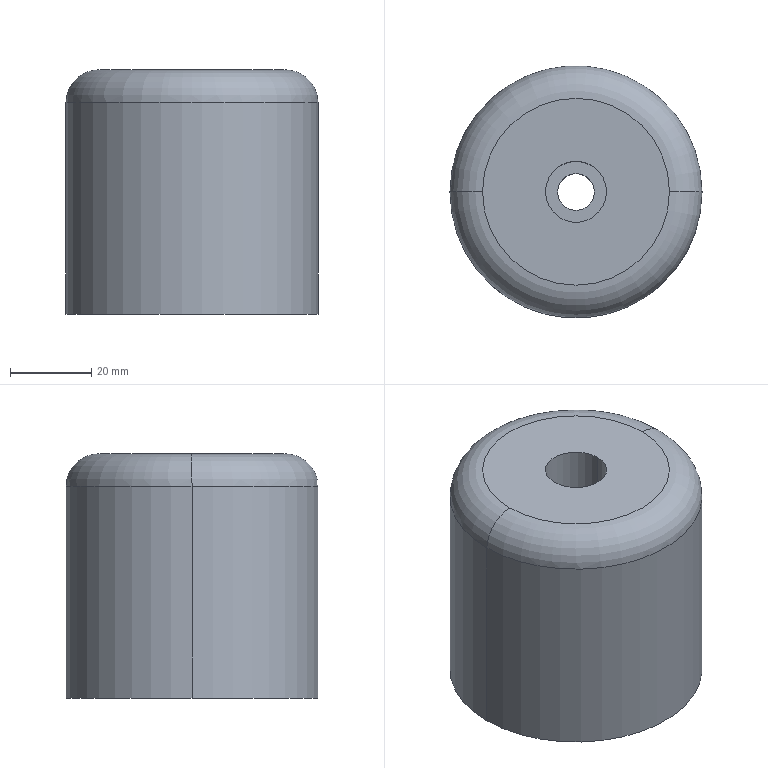Part | STEP file | 1 solid | 19 faces | box 61.9 x 61.9 x 60 mm | volume 168821 mm3 | cylinder 10 | cone 4 | plane 3 | torus 2 | commonest cylinder face diameters 6 x4 9 x2 15 x2 61.9 x2
STEP:
#1=CARTESIAN_POINT('',(0.,0.,0.));
#2=DIRECTION('',(0.,0.,1.));
#3=DIRECTION('',(1.,0.,0.));
#4=AXIS2_PLACEMENT_3D('',#1,#2,#3);
#5=CARTESIAN_POINT('',(-30.95,0.,22.));
#6=VERTEX_POINT('',#5);
#7=CARTESIAN_POINT('',(30.95,0.,22.));
#8=VERTEX_POINT('',#7);
#9=CARTESIAN_POINT('',(0.,0.,22.));
#10=DIRECTION('',(0.,0.,-1.));
#11=DIRECTION('',(1.,0.,0.));
#12=AXIS2_PLACEMENT_3D('',#9,#10,#11);
#13=CIRCLE('',#12,30.95);
#14=CARTESIAN_POINT('',(0.,0.,22.));
#15=DIRECTION('',(0.,0.,1.));
#16=DIRECTION('',(1.,0.,0.));
#17=AXIS2_PLACEMENT_3D('',#14,#15,#16);
#18=TOROIDAL_SURFACE('',#17,22.95,8.);
#19=CARTESIAN_POINT('',(6.283,0.));
#20=DIRECTION('',(-1.,0.));
#21=VECTOR('',#20,1.);
#22=LINE('',#19,#21);
#23=(GEOMETRIC_REPRESENTATION_CONTEXT(2)PARAMETRIC_REPRESENTATION_CONTEXT()REPRESENTATION_CONTEXT('',''));
#24=DEFINITIONAL_REPRESENTATION('',(#22),#23);
#25=PCURVE('',#18,#24);
#26=CARTESIAN_POINT('',(0.,0.,30.));
#27=DIRECTION('',(0.,0.,-1.));
#28=DIRECTION('',(-1.,0.,0.));
#29=AXIS2_PLACEMENT_3D('',#26,#27,#28);
#30=CYLINDRICAL_SURFACE('',#29,30.95);
#31=CARTESIAN_POINT('',(-3.142,8.));
#32=DIRECTION('',(1.,0.));
#33=VECTOR('',#32,1.);
#34=LINE('',#31,#33);
#35=(GEOMETRIC_REPRESENTATION_CONTEXT(2)PARAMETRIC_REPRESENTATION_CONTEXT()REPRESENTATION_CONTEXT('',''));
#36=DEFINITIONAL_REPRESENTATION('',(#34),#35);
#37=PCURVE('',#30,#36);
#38=SURFACE_CURVE('',#13,(#25,#37),.PCURVE_S1.);
#39=EDGE_CURVE('',#6,#8,#38,.T.);
#40=ORIENTED_EDGE('',*,*,#39,.F.);
#41=CARTESIAN_POINT('',(-22.95,0.,30.));
#42=VERTEX_POINT('',#41);
#43=CARTESIAN_POINT('',(-22.95,0.,22.));
#44=DIRECTION('',(0.,1.,0.));
#45=DIRECTION('',(-1.,0.,0.));
#46=AXIS2_PLACEMENT_3D('',#43,#44,#45);
#47=CIRCLE('',#46,8.);
#48=CARTESIAN_POINT('',(3.142,0.));
#49=DIRECTION('',(0.,1.));
#50=VECTOR('',#49,1.);
#51=LINE('',#48,#50);
#52=(GEOMETRIC_REPRESENTATION_CONTEXT(2)PARAMETRIC_REPRESENTATION_CONTEXT()REPRESENTATION_CONTEXT('',''));
#53=DEFINITIONAL_REPRESENTATION('',(#51),#52);
#54=PCURVE('',#18,#53);
#55=CARTESIAN_POINT('',(0.,0.,22.));
#56=DIRECTION('',(0.,0.,1.));
#57=DIRECTION('',(1.,0.,0.));
#58=AXIS2_PLACEMENT_3D('',#55,#56,#57);
#59=TOROIDAL_SURFACE('',#58,22.95,8.);
#60=CARTESIAN_POINT('',(3.142,0.));
#61=DIRECTION('',(0.,1.));
#62=VECTOR('',#61,1.);
#63=LINE('',#60,#62);
#64=(GEOMETRIC_REPRESENTATION_CONTEXT(2)PARAMETRIC_REPRESENTATION_CONTEXT()REPRESENTATION_CONTEXT('',''));
#65=DEFINITIONAL_REPRESENTATION('',(#63),#64);
#66=PCURVE('',#59,#65);
#67=SURFACE_CURVE('',#47,(#54,#66),.PCURVE_S1.);
#68=EDGE_CURVE('',#6,#42,#67,.T.);
#69=ORIENTED_EDGE('',*,*,#68,.T.);
#70=CARTESIAN_POINT('',(22.95,0.,30.));
#71=VERTEX_POINT('',#70);
#72=CARTESIAN_POINT('',(0.,0.,30.));
#73=DIRECTION('',(0.,0.,1.));
#74=DIRECTION('',(1.,0.,0.));
#75=AXIS2_PLACEMENT_3D('',#72,#73,#74);
#76=CIRCLE('',#75,22.95);
#77=CARTESIAN_POINT('',(0.,1.571));
#78=DIRECTION('',(1.,0.));
#79=VECTOR('',#78,1.);
#80=LINE('',#77,#79);
#81=(GEOMETRIC_REPRESENTATION_CONTEXT(2)PARAMETRIC_REPRESENTATION_CONTEXT()REPRESENTATION_CONTEXT('',''));
#82=DEFINITIONAL_REPRESENTATION('',(#80),#81);
#83=PCURVE('',#18,#82);
#84=CARTESIAN_POINT('',(0.,0.,30.));
#85=DIRECTION('',(0.,0.,1.));
#86=DIRECTION('',(1.,0.,0.));
#87=AXIS2_PLACEMENT_3D('',#84,#85,#86);
#88=PLANE('',#87);
#89=CARTESIAN_POINT('',(0.,0.));
#90=DIRECTION('',(1.,0.));
#91=AXIS2_PLACEMENT_2D('',#89,#90);
#92=CIRCLE('',#91,22.95);
#93=(GEOMETRIC_REPRESENTATION_CONTEXT(2)PARAMETRIC_REPRESENTATION_CONTEXT()REPRESENTATION_CONTEXT('',''));
#94=DEFINITIONAL_REPRESENTATION('',(#92),#93);
#95=PCURVE('',#88,#94);
#96=SURFACE_CURVE('',#76,(#83,#95),.PCURVE_S1.);
#97=EDGE_CURVE('',#71,#42,#96,.T.);
#98=ORIENTED_EDGE('',*,*,#97,.F.);
#99=CARTESIAN_POINT('',(22.95,0.,22.));
#100=DIRECTION('',(0.,-1.,0.));
#101=DIRECTION('',(0.,0.,-1.));
#102=AXIS2_PLACEMENT_3D('',#99,#100,#101);
#103=CIRCLE('',#102,8.);
#104=CARTESIAN_POINT('',(0.,-1.571));
#105=DIRECTION('',(0.,1.));
#106=VECTOR('',#105,1.);
#107=LINE('',#104,#106);
#108=(GEOMETRIC_REPRESENTATION_CONTEXT(2)PARAMETRIC_REPRESENTATION_CONTEXT()REPRESENTATION_CONTEXT('',''));
#109=DEFINITIONAL_REPRESENTATION('',(#107),#108);
#110=PCURVE('',#18,#109);
#111=CARTESIAN_POINT('',(6.283,-1.571));
#112=DIRECTION('',(0.,1.));
#113=VECTOR('',#112,1.);
#114=LINE('',#111,#113);
#115=(GEOMETRIC_REPRESENTATION_CONTEXT(2)PARAMETRIC_REPRESENTATION_CONTEXT()REPRESENTATION_CONTEXT('',''));
#116=DEFINITIONAL_REPRESENTATION('',(#114),#115);
#117=PCURVE('',#59,#116);
#118=SURFACE_CURVE('',#103,(#110,#117),.PCURVE_S1.);
#119=EDGE_CURVE('',#8,#71,#118,.T.);
#120=ORIENTED_EDGE('',*,*,#119,.F.);
#121=EDGE_LOOP('',(#40,#69,#98,#120));
#122=FACE_BOUND('',#121,.T.);
#123=ADVANCED_FACE('',(#122),#18,.T.);
#124=CARTESIAN_POINT('',(7.5,0.,-10.));
#125=VERTEX_POINT('',#124);
#126=CARTESIAN_POINT('',(7.5,0.,30.));
#127=VERTEX_POINT('',#126);
#128=CARTESIAN_POINT('',(7.5,0.,30.));
#129=DIRECTION('',(0.,0.,1.));
#130=VECTOR('',#129,1.);
#131=LINE('',#128,#130);
#132=CARTESIAN_POINT('',(0.,0.,30.));
#133=DIRECTION('',(0.,0.,1.));
#134=DIRECTION('',(1.,0.,0.));
#135=AXIS2_PLACEMENT_3D('',#132,#133,#134);
#136=CYLINDRICAL_SURFACE('',#135,7.5);
#137=CARTESIAN_POINT('',(6.283,0.));
#138=DIRECTION('',(0.,1.));
#139=VECTOR('',#138,1.);
#140=LINE('',#137,#139);
#141=(GEOMETRIC_REPRESENTATION_CONTEXT(2)PARAMETRIC_REPRESENTATION_CONTEXT()REPRESENTATION_CONTEXT('',''));
#142=DEFINITIONAL_REPRESENTATION('',(#140),#141);
#143=PCURVE('',#136,#142);
#144=CARTESIAN_POINT('',(0.,0.,30.));
#145=DIRECTION('',(0.,0.,1.));
#146=DIRECTION('',(1.,0.,0.));
#147=AXIS2_PLACEMENT_3D('',#144,#145,#146);
#148=CYLINDRICAL_SURFACE('',#147,7.5);
#149=CARTESIAN_POINT('',(0.,0.));
#150=DIRECTION('',(0.,1.));
#151=VECTOR('',#150,1.);
#152=LINE('',#149,#151);
#153=(GEOMETRIC_REPRESENTATION_CONTEXT(2)PARAMETRIC_REPRESENTATION_CONTEXT()REPRESENTATION_CONTEXT('',''));
#154=DEFINITIONAL_REPRESENTATION('',(#152),#153);
#155=PCURVE('',#148,#154);
#156=SURFACE_CURVE('',#131,(#143,#155),.PCURVE_S1.);
#157=EDGE_CURVE('',#125,#127,#156,.T.);
#158=ORIENTED_EDGE('',*,*,#157,.T.);
#159=CARTESIAN_POINT('',(-7.5,0.,30.));
#160=VERTEX_POINT('',#159);
#161=CARTESIAN_POINT('',(0.,0.,30.));
#162=DIRECTION('',(0.,0.,1.));
#163=DIRECTION('',(1.,0.,0.));
#164=AXIS2_PLACEMENT_3D('',#161,#162,#163);
#165=CIRCLE('',#164,7.5);
#166=CARTESIAN_POINT('',(0.,0.));
#167=DIRECTION('',(1.,0.));
#168=VECTOR('',#167,1.);
#169=LINE('',#166,#168);
#170=(GEOMETRIC_REPRESENTATION_CONTEXT(2)PARAMETRIC_REPRESENTATION_CONTEXT()REPRESENTATION_CONTEXT('',''));
#171=DEFINITIONAL_REPRESENTATION('',(#169),#170);
#172=PCURVE('',#136,#171);
#173=CARTESIAN_POINT('',(0.,0.));
#174=DIRECTION('',(1.,0.));
#175=AXIS2_PLACEMENT_2D('',#173,#174);
#176=CIRCLE('',#175,7.5);
#177=(GEOMETRIC_REPRESENTATION_CONTEXT(2)PARAMETRIC_REPRESENTATION_CONTEXT()REPRESENTATION_CONTEXT('',''));
#178=DEFINITIONAL_REPRESENTATION('',(#176),#177);
#179=PCURVE('',#88,#178);
#180=SURFACE_CURVE('',#165,(#172,#179),.PCURVE_S1.);
#181=EDGE_CURVE('',#160,#127,#180,.T.);
#182=ORIENTED_EDGE('',*,*,#181,.F.);
#183=CARTESIAN_POINT('',(-7.5,0.,-10.));
#184=VERTEX_POINT('',#183);
#185=CARTESIAN_POINT('',(-7.5,0.,30.));
#186=DIRECTION('',(0.,0.,1.));
#187=VECTOR('',#186,1.);
#188=LINE('',#185,#187);
#189=CARTESIAN_POINT('',(3.142,0.));
#190=DIRECTION('',(0.,1.));
#191=VECTOR('',#190,1.);
#192=LINE('',#189,#191);
#193=(GEOMETRIC_REPRESENTATION_CONTEXT(2)PARAMETRIC_REPRESENTATION_CONTEXT()REPRESENTATION_CONTEXT('',''));
#194=DEFINITIONAL_REPRESENTATION('',(#192),#193);
#195=PCURVE('',#136,#194);
#196=CARTESIAN_POINT('',(3.142,0.));
#197=DIRECTION('',(0.,1.));
#198=VECTOR('',#197,1.);
#199=LINE('',#196,#198);
#200=(GEOMETRIC_REPRESENTATION_CONTEXT(2)PARAMETRIC_REPRESENTATION_CONTEXT()REPRESENTATION_CONTEXT('',''));
#201=DEFINITIONAL_REPRESENTATION('',(#199),#200);
#202=PCURVE('',#148,#201);
#203=SURFACE_CURVE('',#188,(#195,#202),.PCURVE_S1.);
#204=EDGE_CURVE('',#184,#160,#203,.T.);
#205=ORIENTED_EDGE('',*,*,#204,.F.);
#206=CARTESIAN_POINT('',(0.,0.,-10.));
#207=DIRECTION('',(0.,0.,1.));
#208=DIRECTION('',(1.,0.,0.));
#209=AXIS2_PLACEMENT_3D('',#206,#207,#208);
#210=CIRCLE('',#209,7.5);
#211=CARTESIAN_POINT('',(0.,-40.));
#212=DIRECTION('',(1.,0.));
#213=VECTOR('',#212,1.);
#214=LINE('',#211,#213);
#215=(GEOMETRIC_REPRESENTATION_CONTEXT(2)PARAMETRIC_REPRESENTATION_CONTEXT()REPRESENTATION_CONTEXT('',''));
#216=DEFINITIONAL_REPRESENTATION('',(#214),#215);
#217=PCURVE('',#136,#216);
#218=CARTESIAN_POINT('',(4.5,0.,-10.));
#219=DIRECTION('',(0.,0.,-1.));
#220=DIRECTION('',(-1.,0.,0.));
#221=AXIS2_PLACEMENT_3D('',#218,#219,#220);
#222=PLANE('',#221);
#223=CARTESIAN_POINT('',(-3.,0.));
#224=CARTESIAN_POINT('',(-3.,12.99));
#225=CARTESIAN_POINT('',(8.25,6.495));
#226=CARTESIAN_POINT('',(19.5,0.));
#227=CARTESIAN_POINT('',(8.25,-6.495));
#228=CARTESIAN_POINT('',(-3.,-12.99));
#229=CARTESIAN_POINT('',(-3.,0.));
#230=(BOUNDED_CURVE()B_SPLINE_CURVE(2,(#223,#224,#225,#226,#227,#228,#229),.UNSPECIFIED.,.T.,.F.)B_SPLINE_CURVE_WITH_KNOTS((1,2,2,2,2,1),(-2.094,0.,2.094,4.189,6.283,8.378),.UNSPECIFIED.)CURVE()GEOMETRIC_REPRESENTATION_ITEM()RATIONAL_B_SPLINE_CURVE((1.,0.5,1.,0.5,1.,0.5,1.))REPRESENTATION_ITEM(''));
#231=(GEOMETRIC_REPRESENTATION_CONTEXT(2)PARAMETRIC_REPRESENTATION_CONTEXT()REPRESENTATION_CONTEXT('',''));
#232=DEFINITIONAL_REPRESENTATION('',(#230),#231);
#233=PCURVE('',#222,#232);
#234=SURFACE_CURVE('',#210,(#217,#233),.PCURVE_S1.);
#235=EDGE_CURVE('',#184,#125,#234,.T.);
#236=ORIENTED_EDGE('',*,*,#235,.T.);
#237=EDGE_LOOP('',(#158,#182,#205,#236));
#238=FACE_BOUND('',#237,.F.);
#239=ADVANCED_FACE('',(#238),#136,.F.);
#240=CARTESIAN_POINT('',(4.5,0.,-30.));
#241=VERTEX_POINT('',#240);
#242=CARTESIAN_POINT('',(4.5,0.,-10.));
#243=VERTEX_POINT('',#242);
#244=CARTESIAN_POINT('',(4.5,0.,30.));
#245=DIRECTION('',(0.,0.,1.));
#246=VECTOR('',#245,1.);
#247=LINE('',#244,#246);
#248=CARTESIAN_POINT('',(0.,0.,30.));
#249=DIRECTION('',(0.,0.,1.));
#250=DIRECTION('',(1.,0.,0.));
#251=AXIS2_PLACEMENT_3D('',#248,#249,#250);
#252=CYLINDRICAL_SURFACE('',#251,4.5);
#253=CARTESIAN_POINT('',(6.283,0.));
#254=DIRECTION('',(0.,1.));
#255=VECTOR('',#254,1.);
#256=LINE('',#253,#255);
#257=(GEOMETRIC_REPRESENTATION_CONTEXT(2)PARAMETRIC_REPRESENTATION_CONTEXT()REPRESENTATION_CONTEXT('',''));
#258=DEFINITIONAL_REPRESENTATION('',(#256),#257);
#259=PCURVE('',#252,#258);
#260=CARTESIAN_POINT('',(0.,0.,30.));
#261=DIRECTION('',(0.,0.,1.));
#262=DIRECTION('',(1.,0.,0.));
#263=AXIS2_PLACEMENT_3D('',#260,#261,#262);
#264=CYLINDRICAL_SURFACE('',#263,4.5);
#265=CARTESIAN_POINT('',(0.,0.));
#266=DIRECTION('',(0.,1.));
#267=VECTOR('',#266,1.);
#268=LINE('',#265,#267);
#269=(GEOMETRIC_REPRESENTATION_CONTEXT(2)PARAMETRIC_REPRESENTATION_CONTEXT()REPRESENTATION_CONTEXT('',''));
#270=DEFINITIONAL_REPRESENTATION('',(#268),#269);
#271=PCURVE('',#264,#270);
#272=SURFACE_CURVE('',#247,(#259,#271),.PCURVE_S1.);
#273=EDGE_CURVE('',#241,#243,#272,.T.);
#274=ORIENTED_EDGE('',*,*,#273,.T.);
#275=CARTESIAN_POINT('',(-4.5,0.,-10.));
#276=VERTEX_POINT('',#275);
#277=CARTESIAN_POINT('',(0.,0.,-10.));
#278=DIRECTION('',(0.,0.,1.));
#279=DIRECTION('',(1.,0.,0.));
#280=AXIS2_PLACEMENT_3D('',#277,#278,#279);
#281=CIRCLE('',#280,4.5);
#282=CARTESIAN_POINT('',(0.,-40.));
#283=DIRECTION('',(1.,0.));
#284=VECTOR('',#283,1.);
#285=LINE('',#282,#284);
#286=(GEOMETRIC_REPRESENTATION_CONTEXT(2)PARAMETRIC_REPRESENTATION_CONTEXT()REPRESENTATION_CONTEXT('',''));
#287=DEFINITIONAL_REPRESENTATION('',(#285),#286);
#288=PCURVE('',#252,#287);
#289=CARTESIAN_POINT('',(0.,0.));
#290=CARTESIAN_POINT('',(0.,7.794));
#291=CARTESIAN_POINT('',(6.75,3.897));
#292=CARTESIAN_POINT('',(13.5,0.));
#293=CARTESIAN_POINT('',(6.75,-3.897));
#294=CARTESIAN_POINT('',(0.,-7.794));
#295=CARTESIAN_POINT('',(0.,0.));
#296=(BOUNDED_CURVE()B_SPLINE_CURVE(2,(#289,#290,#291,#292,#293,#294,#295),.UNSPECIFIED.,.T.,.F.)B_SPLINE_CURVE_WITH_KNOTS((1,2,2,2,2,1),(-2.094,0.,2.094,4.189,6.283,8.378),.UNSPECIFIED.)CURVE()GEOMETRIC_REPRESENTATION_ITEM()RATIONAL_B_SPLINE_CURVE((1.,0.5,1.,0.5,1.,0.5,1.))REPRESENTATION_ITEM(''));
#297=(GEOMETRIC_REPRESENTATION_CONTEXT(2)PARAMETRIC_REPRESENTATION_CONTEXT()REPRESENTATION_CONTEXT('',''));
#298=DEFINITIONAL_REPRESENTATION('',(#296),#297);
#299=PCURVE('',#222,#298);
#300=SURFACE_CURVE('',#281,(#288,#299),.PCURVE_S1.);
#301=EDGE_CURVE('',#276,#243,#300,.T.);
#302=ORIENTED_EDGE('',*,*,#301,.F.);
#303=CARTESIAN_POINT('',(-4.5,0.,-30.));
#304=VERTEX_POINT('',#303);
#305=CARTESIAN_POINT('',(-4.5,0.,30.));
#306=DIRECTION('',(0.,0.,1.));
#307=VECTOR('',#306,1.);
#308=LINE('',#305,#307);
#309=CARTESIAN_POINT('',(3.142,0.));
#310=DIRECTION('',(0.,1.));
#311=VECTOR('',#310,1.);
#312=LINE('',#309,#311);
#313=(GEOMETRIC_REPRESENTATION_CONTEXT(2)PARAMETRIC_REPRESENTATION_CONTEXT()REPRESENTATION_CONTEXT('',''));
#314=DEFINITIONAL_REPRESENTATION('',(#312),#313);
#315=PCURVE('',#252,#314);
#316=CARTESIAN_POINT('',(3.142,0.));
#317=DIRECTION('',(0.,1.));
#318=VECTOR('',#317,1.);
#319=LINE('',#316,#318);
#320=(GEOMETRIC_REPRESENTATION_CONTEXT(2)PARAMETRIC_REPRESENTATION_CONTEXT()REPRESENTATION_CONTEXT('',''));
#321=DEFINITIONAL_REPRESENTATION('',(#319),#320);
#322=PCURVE('',#264,#321);
#323=SURFACE_CURVE('',#308,(#315,#322),.PCURVE_S1.);
#324=EDGE_CURVE('',#304,#276,#323,.T.);
#325=ORIENTED_EDGE('',*,*,#324,.F.);
#326=CARTESIAN_POINT('',(0.,0.,-30.));
#327=DIRECTION('',(0.,0.,1.));
#328=DIRECTION('',(1.,0.,0.));
#329=AXIS2_PLACEMENT_3D('',#326,#327,#328);
#330=CIRCLE('',#329,4.5);
#331=CARTESIAN_POINT('',(0.,-60.));
#332=DIRECTION('',(1.,0.));
#333=VECTOR('',#332,1.);
#334=LINE('',#331,#333);
#335=(GEOMETRIC_REPRESENTATION_CONTEXT(2)PARAMETRIC_REPRESENTATION_CONTEXT()REPRESENTATION_CONTEXT('',''));
#336=DEFINITIONAL_REPRESENTATION('',(#334),#335);
#337=PCURVE('',#252,#336);
#338=CARTESIAN_POINT('',(0.,0.,-30.));
#339=DIRECTION('',(0.,0.,1.));
#340=DIRECTION('',(1.,0.,0.));
#341=AXIS2_PLACEMENT_3D('',#338,#339,#340);
#342=PLANE('',#341);
#343=CARTESIAN_POINT('',(0.,0.));
#344=DIRECTION('',(1.,0.));
#345=AXIS2_PLACEMENT_2D('',#343,#344);
#346=CIRCLE('',#345,4.5);
#347=(GEOMETRIC_REPRESENTATION_CONTEXT(2)PARAMETRIC_REPRESENTATION_CONTEXT()REPRESENTATION_CONTEXT('',''));
#348=DEFINITIONAL_REPRESENTATION('',(#346),#347);
#349=PCURVE('',#342,#348);
#350=SURFACE_CURVE('',#330,(#337,#349),.PCURVE_S1.);
#351=EDGE_CURVE('',#304,#241,#350,.T.);
#352=ORIENTED_EDGE('',*,*,#351,.T.);
#353=EDGE_LOOP('',(#274,#302,#325,#352));
#354=FACE_BOUND('',#353,.F.);
#355=ADVANCED_FACE('',(#354),#252,.F.);
#356=CARTESIAN_POINT('',(17.,0.,-15.));
#357=VERTEX_POINT('',#356);
#358=CARTESIAN_POINT('',(17.,0.,-30.));
#359=VERTEX_POINT('',#358);
#360=CARTESIAN_POINT('',(17.,0.,-30.));
#361=DIRECTION('',(0.,0.,-1.));
#362=VECTOR('',#361,1.);
#363=LINE('',#360,#362);
#364=CARTESIAN_POINT('',(20.,0.,-30.));
#365=DIRECTION('',(0.,0.,-1.));
#366=DIRECTION('',(-1.,0.,0.));
#367=AXIS2_PLACEMENT_3D('',#364,#365,#366);
#368=CYLINDRICAL_SURFACE('',#367,3.);
#369=CARTESIAN_POINT('',(6.283,0.));
#370=DIRECTION('',(0.,1.));
#371=VECTOR('',#370,1.);
#372=LINE('',#369,#371);
#373=(GEOMETRIC_REPRESENTATION_CONTEXT(2)PARAMETRIC_REPRESENTATION_CONTEXT()REPRESENTATION_CONTEXT('',''));
#374=DEFINITIONAL_REPRESENTATION('',(#372),#373);
#375=PCURVE('',#368,#374);
#376=CARTESIAN_POINT('',(20.,0.,-30.));
#377=DIRECTION('',(0.,0.,-1.));
#378=DIRECTION('',(-1.,0.,0.));
#379=AXIS2_PLACEMENT_3D('',#376,#377,#378);
#380=CYLINDRICAL_SURFACE('',#379,3.);
#381=CARTESIAN_POINT('',(0.,0.));
#382=DIRECTION('',(0.,1.));
#383=VECTOR('',#382,1.);
#384=LINE('',#381,#383);
#385=(GEOMETRIC_REPRESENTATION_CONTEXT(2)PARAMETRIC_REPRESENTATION_CONTEXT()REPRESENTATION_CONTEXT('',''));
#386=DEFINITIONAL_REPRESENTATION('',(#384),#385);
#387=PCURVE('',#380,#386);
#388=SURFACE_CURVE('',#363,(#375,#387),.PCURVE_S1.);
#389=EDGE_CURVE('',#357,#359,#388,.T.);
#390=ORIENTED_EDGE('',*,*,#389,.T.);
#391=CARTESIAN_POINT('',(23.,0.,-30.));
#392=VERTEX_POINT('',#391);
#393=CARTESIAN_POINT('',(20.,0.,-30.));
#394=DIRECTION('',(0.,0.,-1.));
#395=DIRECTION('',(-1.,0.,0.));
#396=AXIS2_PLACEMENT_3D('',#393,#394,#395);
#397=CIRCLE('',#396,3.);
#398=CARTESIAN_POINT('',(0.,0.));
#399=DIRECTION('',(1.,0.));
#400=VECTOR('',#399,1.);
#401=LINE('',#398,#400);
#402=(GEOMETRIC_REPRESENTATION_CONTEXT(2)PARAMETRIC_REPRESENTATION_CONTEXT()REPRESENTATION_CONTEXT('',''));
#403=DEFINITIONAL_REPRESENTATION('',(#401),#402);
#404=PCURVE('',#368,#403);
#405=CARTESIAN_POINT('',(17.,0.));
#406=CARTESIAN_POINT('',(17.,5.196));
#407=CARTESIAN_POINT('',(21.5,2.598));
#408=CARTESIAN_POINT('',(26.,0.));
#409=CARTESIAN_POINT('',(21.5,-2.598));
#410=CARTESIAN_POINT('',(17.,-5.196));
#411=CARTESIAN_POINT('',(17.,0.));
#412=(BOUNDED_CURVE()B_SPLINE_CURVE(2,(#405,#406,#407,#408,#409,#410,#411),.UNSPECIFIED.,.T.,.F.)B_SPLINE_CURVE_WITH_KNOTS((1,2,2,2,2,1),(-2.094,0.,2.094,4.189,6.283,8.378),.UNSPECIFIED.)CURVE()GEOMETRIC_REPRESENTATION_ITEM()RATIONAL_B_SPLINE_CURVE((1.,0.5,1.,0.5,1.,0.5,1.))REPRESENTATION_ITEM(''));
#413=(GEOMETRIC_REPRESENTATION_CONTEXT(2)PARAMETRIC_REPRESENTATION_CONTEXT()REPRESENTATION_CONTEXT('',''));
#414=DEFINITIONAL_REPRESENTATION('',(#412),#413);
#415=PCURVE('',#342,#414);
#416=SURFACE_CURVE('',#397,(#404,#415),.PCURVE_S1.);
#417=EDGE_CURVE('',#392,#359,#416,.T.);
#418=ORIENTED_EDGE('',*,*,#417,.F.);
#419=CARTESIAN_POINT('',(23.,0.,-15.));
#420=VERTEX_POINT('',#419);
#421=CARTESIAN_POINT('',(23.,0.,-30.));
#422=DIRECTION('',(0.,0.,-1.));
#423=VECTOR('',#422,1.);
#424=LINE('',#421,#423);
#425=CARTESIAN_POINT('',(3.142,0.));
#426=DIRECTION('',(0.,1.));
#427=VECTOR('',#426,1.);
#428=LINE('',#425,#427);
#429=(GEOMETRIC_REPRESENTATION_CONTEXT(2)PARAMETRIC_REPRESENTATION_CONTEXT()REPRESENTATION_CONTEXT('',''));
#430=DEFINITIONAL_REPRESENTATION('',(#428),#429);
#431=PCURVE('',#368,#430);
#432=CARTESIAN_POINT('',(3.142,0.));
#433=DIRECTION('',(0.,1.));
#434=VECTOR('',#433,1.);
#435=LINE('',#432,#434);
#436=(GEOMETRIC_REPRESENTATION_CONTEXT(2)PARAMETRIC_REPRESENTATION_CONTEXT()REPRESENTATION_CONTEXT('',''));
#437=DEFINITIONAL_REPRESENTATION('',(#435),#436);
#438=PCURVE('',#380,#437);
#439=SURFACE_CURVE('',#424,(#431,#438),.PCURVE_S1.);
#440=EDGE_CURVE('',#420,#392,#439,.T.);
#441=ORIENTED_EDGE('',*,*,#440,.F.);
#442=CARTESIAN_POINT('',(20.,0.,-15.));
#443=DIRECTION('',(0.,0.,-1.));
#444=DIRECTION('',(-1.,0.,0.));
#445=AXIS2_PLACEMENT_3D('',#442,#443,#444);
#446=CIRCLE('',#445,3.);
#447=CARTESIAN_POINT('',(0.,-15.));
#448=DIRECTION('',(1.,0.));
#449=VECTOR('',#448,1.);
#450=LINE('',#447,#449);
#451=(GEOMETRIC_REPRESENTATION_CONTEXT(2)PARAMETRIC_REPRESENTATION_CONTEXT()REPRESENTATION_CONTEXT('',''));
#452=DEFINITIONAL_REPRESENTATION('',(#450),#451);
#453=PCURVE('',#368,#452);
#454=CARTESIAN_POINT('',(20.,0.,-15.));
#455=DIRECTION('',(0.,0.,-1.));
#456=DIRECTION('',(-1.,0.,0.));
#457=AXIS2_PLACEMENT_3D('',#454,#455,#456);
#458=CONICAL_SURFACE('',#457,3.,1.03);
#459=CARTESIAN_POINT('',(0.,0.));
#460=DIRECTION('',(1.,0.));
#461=VECTOR('',#460,1.);
#462=LINE('',#459,#461);
#463=(GEOMETRIC_REPRESENTATION_CONTEXT(2)PARAMETRIC_REPRESENTATION_CONTEXT()REPRESENTATION_CONTEXT('',''));
#464=DEFINITIONAL_REPRESENTATION('',(#462),#463);
#465=PCURVE('',#458,#464);
#466=SURFACE_CURVE('',#446,(#453,#465),.PCURVE_S1.);
#467=EDGE_CURVE('',#420,#357,#466,.T.);
#468=ORIENTED_EDGE('',*,*,#467,.T.);
#469=EDGE_LOOP('',(#390,#418,#441,#468));
#470=FACE_BOUND('',#469,.F.);
#471=ADVANCED_FACE('',(#470),#368,.F.);
#472=ORIENTED_EDGE('',*,*,#467,.F.);
#473=CARTESIAN_POINT('',(20.,0.,-13.197));
#474=VERTEX_POINT('',#473);
#475=CARTESIAN_POINT('',(23.,0.,-15.));
#476=DIRECTION('',(0.8572,0.,-0.515));
#477=VECTOR('',#476,1.);
#478=LINE('',#475,#477);
#479=CARTESIAN_POINT('',(3.142,-1.803));
#480=CARTESIAN_POINT('',(3.142,-1.775));
#481=CARTESIAN_POINT('',(3.142,-1.721));
#482=CARTESIAN_POINT('',(3.142,-1.639));
#483=CARTESIAN_POINT('',(3.142,-1.557));
#484=CARTESIAN_POINT('',(3.142,-1.475));
#485=CARTESIAN_POINT('',(3.142,-1.393));
#486=CARTESIAN_POINT('',(3.142,-1.311));
#487=CARTESIAN_POINT('',(3.142,-1.229));
#488=CARTESIAN_POINT('',(3.142,-1.147));
#489=CARTESIAN_POINT('',(3.142,-1.065));
#490=CARTESIAN_POINT('',(3.142,-0.9832));
#491=CARTESIAN_POINT('',(3.142,-0.9013));
#492=CARTESIAN_POINT('',(3.142,-0.8194));
#493=CARTESIAN_POINT('',(3.142,-0.7374));
#494=CARTESIAN_POINT('',(3.142,-0.6555));
#495=CARTESIAN_POINT('',(3.142,-0.5735));
#496=CARTESIAN_POINT('',(3.142,-0.4916));
#497=CARTESIAN_POINT('',(3.142,-0.4097));
#498=CARTESIAN_POINT('',(3.142,-0.3277));
#499=CARTESIAN_POINT('',(3.142,-0.2458));
#500=CARTESIAN_POINT('',(3.142,-0.1639));
#501=CARTESIAN_POINT('',(3.142,-0.08194));
#502=CARTESIAN_POINT('',(3.142,-0.02731));
#503=CARTESIAN_POINT('',(3.142,0.));
#504=B_SPLINE_CURVE_WITH_KNOTS('',3,(#479,#480,#481,#482,#483,#484,#485,#486,#487,#488,#489,#490,#491,#492,#493,#494,#495,#496,#497,#498,#499,#500,#501,#502,#503),.UNSPECIFIED.,.F.,.F.,(4,1,1,1,1,1,1,1,1,1,1,1,1,1,1,1,1,1,1,1,1,1,4),(-3.5,-3.341,-3.182,-3.023,-2.864,-2.704,-2.545,-2.386,-2.227,-2.068,-1.909,-1.75,-1.591,-1.432,-1.273,-1.114,-0.9545,-0.7954,-0.6363,-0.4773,-0.3182,-0.1591,0.),.UNSPECIFIED.);
#505=(GEOMETRIC_REPRESENTATION_CONTEXT(2)PARAMETRIC_REPRESENTATION_CONTEXT()REPRESENTATION_CONTEXT('',''));
#506=DEFINITIONAL_REPRESENTATION('',(#504),#505);
#507=PCURVE('',#458,#506);
#508=CARTESIAN_POINT('',(20.,0.,-15.));
#509=DIRECTION('',(0.,0.,-1.));
#510=DIRECTION('',(-1.,0.,0.));
#511=AXIS2_PLACEMENT_3D('',#508,#509,#510);
#512=CONICAL_SURFACE('',#511,3.,1.03);
#513=CARTESIAN_POINT('',(3.142,-1.803));
#514=CARTESIAN_POINT('',(3.142,-1.775));
#515=CARTESIAN_POINT('',(3.142,-1.721));
#516=CARTESIAN_POINT('',(3.142,-1.639));
#517=CARTESIAN_POINT('',(3.142,-1.557));
#518=CARTESIAN_POINT('',(3.142,-1.475));
#519=CARTESIAN_POINT('',(3.142,-1.393));
#520=CARTESIAN_POINT('',(3.142,-1.311));
#521=CARTESIAN_POINT('',(3.142,-1.229));
#522=CARTESIAN_POINT('',(3.142,-1.147));
#523=CARTESIAN_POINT('',(3.142,-1.065));
#524=CARTESIAN_POINT('',(3.142,-0.9832));
#525=CARTESIAN_POINT('',(3.142,-0.9013));
#526=CARTESIAN_POINT('',(3.142,-0.8194));
#527=CARTESIAN_POINT('',(3.142,-0.7374));
#528=CARTESIAN_POINT('',(3.142,-0.6555));
#529=CARTESIAN_POINT('',(3.142,-0.5735));
#530=CARTESIAN_POINT('',(3.142,-0.4916));
#531=CARTESIAN_POINT('',(3.142,-0.4097));
#532=CARTESIAN_POINT('',(3.142,-0.3277));
#533=CARTESIAN_POINT('',(3.142,-0.2458));
#534=CARTESIAN_POINT('',(3.142,-0.1639));
#535=CARTESIAN_POINT('',(3.142,-0.08194));
#536=CARTESIAN_POINT('',(3.142,-0.02731));
#537=CARTESIAN_POINT('',(3.142,0.));
#538=B_SPLINE_CURVE_WITH_KNOTS('',3,(#513,#514,#515,#516,#517,#518,#519,#520,#521,#522,#523,#524,#525,#526,#527,#528,#529,#530,#531,#532,#533,#534,#535,#536,#537),.UNSPECIFIED.,.F.,.F.,(4,1,1,1,1,1,1,1,1,1,1,1,1,1,1,1,1,1,1,1,1,1,4),(-3.5,-3.341,-3.182,-3.023,-2.864,-2.704,-2.545,-2.386,-2.227,-2.068,-1.909,-1.75,-1.591,-1.432,-1.273,-1.114,-0.9545,-0.7954,-0.6363,-0.4773,-0.3182,-0.1591,0.),.UNSPECIFIED.);
#539=(GEOMETRIC_REPRESENTATION_CONTEXT(2)PARAMETRIC_REPRESENTATION_CONTEXT()REPRESENTATION_CONTEXT('',''));
#540=DEFINITIONAL_REPRESENTATION('',(#538),#539);
#541=PCURVE('',#512,#540);
#542=SURFACE_CURVE('',#478,(#507,#541),.PCURVE_S1.);
#543=EDGE_CURVE('',#474,#420,#542,.T.);
#544=ORIENTED_EDGE('',*,*,#543,.F.);
#545=CARTESIAN_POINT('',(17.,0.,-15.));
#546=DIRECTION('',(-0.8572,0.,-0.515));
#547=VECTOR('',#546,1.);
#548=LINE('',#545,#547);
#549=CARTESIAN_POINT('',(6.283,0.));
#550=DIRECTION('',(0.,1.));
#551=VECTOR('',#550,1.);
#552=LINE('',#549,#551);
#553=(GEOMETRIC_REPRESENTATION_CONTEXT(2)PARAMETRIC_REPRESENTATION_CONTEXT()REPRESENTATION_CONTEXT('',''));
#554=DEFINITIONAL_REPRESENTATION('',(#552),#553);
#555=PCURVE('',#458,#554);
#556=CARTESIAN_POINT('',(0.,0.));
#557=DIRECTION('',(0.,1.));
#558=VECTOR('',#557,1.);
#559=LINE('',#556,#558);
#560=(GEOMETRIC_REPRESENTATION_CONTEXT(2)PARAMETRIC_REPRESENTATION_CONTEXT()REPRESENTATION_CONTEXT('',''));
#561=DEFINITIONAL_REPRESENTATION('',(#559),#560);
#562=PCURVE('',#512,#561);
#563=SURFACE_CURVE('',#548,(#555,#562),.PCURVE_S1.);
#564=EDGE_CURVE('',#474,#357,#563,.T.);
#565=ORIENTED_EDGE('',*,*,#564,.T.);
#566=EDGE_LOOP('',(#472,#544,#565));
#567=FACE_BOUND('',#566,.F.);
#568=ADVANCED_FACE('',(#567),#458,.F.);
#569=CARTESIAN_POINT('',(-23.,0.,-15.));
#570=VERTEX_POINT('',#569);
#571=CARTESIAN_POINT('',(-23.,0.,-30.));
#572=VERTEX_POINT('',#571);
#573=CARTESIAN_POINT('',(-23.,0.,-30.));
#574=DIRECTION('',(0.,0.,-1.));
#575=VECTOR('',#574,1.);
#576=LINE('',#573,#575);
#577=CARTESIAN_POINT('',(-20.,0.,-30.));
#578=DIRECTION('',(0.,0.,-1.));
#579=DIRECTION('',(-1.,0.,0.));
#580=AXIS2_PLACEMENT_3D('',#577,#578,#579);
#581=CYLINDRICAL_SURFACE('',#580,3.);
#582=CARTESIAN_POINT('',(6.283,0.));
#583=DIRECTION('',(0.,1.));
#584=VECTOR('',#583,1.);
#585=LINE('',#582,#584);
#586=(GEOMETRIC_REPRESENTATION_CONTEXT(2)PARAMETRIC_REPRESENTATION_CONTEXT()REPRESENTATION_CONTEXT('',''));
#587=DEFINITIONAL_REPRESENTATION('',(#585),#586);
#588=PCURVE('',#581,#587);
#589=CARTESIAN_POINT('',(-20.,0.,-30.));
#590=DIRECTION('',(0.,0.,-1.));
#591=DIRECTION('',(-1.,0.,0.));
#592=AXIS2_PLACEMENT_3D('',#589,#590,#591);
#593=CYLINDRICAL_SURFACE('',#592,3.);
#594=CARTESIAN_POINT('',(0.,0.));
#595=DIRECTION('',(0.,1.));
#596=VECTOR('',#595,1.);
#597=LINE('',#594,#596);
#598=(GEOMETRIC_REPRESENTATION_CONTEXT(2)PARAMETRIC_REPRESENTATION_CONTEXT()REPRESENTATION_CONTEXT('',''));
#599=DEFINITIONAL_REPRESENTATION('',(#597),#598);
#600=PCURVE('',#593,#599);
#601=SURFACE_CURVE('',#576,(#588,#600),.PCURVE_S1.);
#602=EDGE_CURVE('',#570,#572,#601,.T.);
#603=ORIENTED_EDGE('',*,*,#602,.T.);
#604=CARTESIAN_POINT('',(-17.,0.,-30.));
#605=VERTEX_POINT('',#604);
#606=CARTESIAN_POINT('',(-20.,0.,-30.));
#607=DIRECTION('',(0.,0.,-1.));
#608=DIRECTION('',(-1.,0.,0.));
#609=AXIS2_PLACEMENT_3D('',#606,#607,#608);
#610=CIRCLE('',#609,3.);
#611=CARTESIAN_POINT('',(0.,0.));
#612=DIRECTION('',(1.,0.));
#613=VECTOR('',#612,1.);
#614=LINE('',#611,#613);
#615=(GEOMETRIC_REPRESENTATION_CONTEXT(2)PARAMETRIC_REPRESENTATION_CONTEXT()REPRESENTATION_CONTEXT('',''));
#616=DEFINITIONAL_REPRESENTATION('',(#614),#615);
#617=PCURVE('',#581,#616);
#618=CARTESIAN_POINT('',(-23.,0.));
#619=CARTESIAN_POINT('',(-23.,5.196));
#620=CARTESIAN_POINT('',(-18.5,2.598));
#621=CARTESIAN_POINT('',(-14.,0.));
#622=CARTESIAN_POINT('',(-18.5,-2.598));
#623=CARTESIAN_POINT('',(-23.,-5.196));
#624=CARTESIAN_POINT('',(-23.,0.));
#625=(BOUNDED_CURVE()B_SPLINE_CURVE(2,(#618,#619,#620,#621,#622,#623,#624),.UNSPECIFIED.,.T.,.F.)B_SPLINE_CURVE_WITH_KNOTS((1,2,2,2,2,1),(-2.094,0.,2.094,4.189,6.283,8.378),.UNSPECIFIED.)CURVE()GEOMETRIC_REPRESENTATION_ITEM()RATIONAL_B_SPLINE_CURVE((1.,0.5,1.,0.5,1.,0.5,1.))REPRESENTATION_ITEM(''));
#626=(GEOMETRIC_REPRESENTATION_CONTEXT(2)PARAMETRIC_REPRESENTATION_CONTEXT()REPRESENTATION_CONTEXT('',''));
#627=DEFINITIONAL_REPRESENTATION('',(#625),#626);
#628=PCURVE('',#342,#627);
#629=SURFACE_CURVE('',#610,(#617,#628),.PCURVE_S1.);
#630=EDGE_CURVE('',#605,#572,#629,.T.);
#631=ORIENTED_EDGE('',*,*,#630,.F.);
#632=CARTESIAN_POINT('',(-17.,0.,-15.));
#633=VERTEX_POINT('',#632);
#634=CARTESIAN_POINT('',(-17.,0.,-30.));
#635=DIRECTION('',(0.,0.,-1.));
#636=VECTOR('',#635,1.);
#637=LINE('',#634,#636);
#638=CARTESIAN_POINT('',(3.142,0.));
#639=DIRECTION('',(0.,1.));
#640=VECTOR('',#639,1.);
#641=LINE('',#638,#640);
#642=(GEOMETRIC_REPRESENTATION_CONTEXT(2)PARAMETRIC_REPRESENTATION_CONTEXT()REPRESENTATION_CONTEXT('',''));
#643=DEFINITIONAL_REPRESENTATION('',(#641),#642);
#644=PCURVE('',#581,#643);
#645=CARTESIAN_POINT('',(3.142,0.));
#646=DIRECTION('',(0.,1.));
#647=VECTOR('',#646,1.);
#648=LINE('',#645,#647);
#649=(GEOMETRIC_REPRESENTATION_CONTEXT(2)PARAMETRIC_REPRESENTATION_CONTEXT()REPRESENTATION_CONTEXT('',''));
#650=DEFINITIONAL_REPRESENTATION('',(#648),#649);
#651=PCURVE('',#593,#650);
#652=SURFACE_CURVE('',#637,(#644,#651),.PCURVE_S1.);
#653=EDGE_CURVE('',#633,#605,#652,.T.);
#654=ORIENTED_EDGE('',*,*,#653,.F.);
#655=CARTESIAN_POINT('',(-20.,0.,-15.));
#656=DIRECTION('',(0.,0.,-1.));
#657=DIRECTION('',(-1.,0.,0.));
#658=AXIS2_PLACEMENT_3D('',#655,#656,#657);
#659=CIRCLE('',#658,3.);
#660=CARTESIAN_POINT('',(0.,-15.));
#661=DIRECTION('',(1.,0.));
#662=VECTOR('',#661,1.);
#663=LINE('',#660,#662);
#664=(GEOMETRIC_REPRESENTATION_CONTEXT(2)PARAMETRIC_REPRESENTATION_CONTEXT()REPRESENTATION_CONTEXT('',''));
#665=DEFINITIONAL_REPRESENTATION('',(#663),#664);
#666=PCURVE('',#581,#665);
#667=CARTESIAN_POINT('',(-20.,0.,-15.));
#668=DIRECTION('',(0.,0.,-1.));
#669=DIRECTION('',(-1.,0.,0.));
#670=AXIS2_PLACEMENT_3D('',#667,#668,#669);
#671=CONICAL_SURFACE('',#670,3.,1.03);
#672=CARTESIAN_POINT('',(0.,0.));
#673=DIRECTION('',(1.,0.));
#674=VECTOR('',#673,1.);
#675=LINE('',#672,#674);
#676=(GEOMETRIC_REPRESENTATION_CONTEXT(2)PARAMETRIC_REPRESENTATION_CONTEXT()REPRESENTATION_CONTEXT('',''));
#677=DEFINITIONAL_REPRESENTATION('',(#675),#676);
#678=PCURVE('',#671,#677);
#679=SURFACE_CURVE('',#659,(#666,#678),.PCURVE_S1.);
#680=EDGE_CURVE('',#633,#570,#679,.T.);
#681=ORIENTED_EDGE('',*,*,#680,.T.);
#682=EDGE_LOOP('',(#603,#631,#654,#681));
#683=FACE_BOUND('',#682,.F.);
#684=ADVANCED_FACE('',(#683),#581,.F.);
#685=ORIENTED_EDGE('',*,*,#680,.F.);
#686=CARTESIAN_POINT('',(-20.,0.,-13.197));
#687=VERTEX_POINT('',#686);
#688=CARTESIAN_POINT('',(-17.,0.,-15.));
#689=DIRECTION('',(0.8572,0.,-0.515));
#690=VECTOR('',#689,1.);
#691=LINE('',#688,#690);
#692=CARTESIAN_POINT('',(3.142,-1.803));
#693=CARTESIAN_POINT('',(3.142,-1.775));
#694=CARTESIAN_POINT('',(3.142,-1.721));
#695=CARTESIAN_POINT('',(3.142,-1.639));
#696=CARTESIAN_POINT('',(3.142,-1.557));
#697=CARTESIAN_POINT('',(3.142,-1.475));
#698=CARTESIAN_POINT('',(3.142,-1.393));
#699=CARTESIAN_POINT('',(3.142,-1.311));
#700=CARTESIAN_POINT('',(3.142,-1.229));
#701=CARTESIAN_POINT('',(3.142,-1.147));
#702=CARTESIAN_POINT('',(3.142,-1.065));
#703=CARTESIAN_POINT('',(3.142,-0.9832));
#704=CARTESIAN_POINT('',(3.142,-0.9013));
#705=CARTESIAN_POINT('',(3.142,-0.8194));
#706=CARTESIAN_POINT('',(3.142,-0.7374));
#707=CARTESIAN_POINT('',(3.142,-0.6555));
#708=CARTESIAN_POINT('',(3.142,-0.5735));
#709=CARTESIAN_POINT('',(3.142,-0.4916));
#710=CARTESIAN_POINT('',(3.142,-0.4097));
#711=CARTESIAN_POINT('',(3.142,-0.3277));
#712=CARTESIAN_POINT('',(3.142,-0.2458));
#713=CARTESIAN_POINT('',(3.142,-0.1639));
#714=CARTESIAN_POINT('',(3.142,-0.08194));
#715=CARTESIAN_POINT('',(3.142,-0.02731));
#716=CARTESIAN_POINT('',(3.142,0.));
#717=B_SPLINE_CURVE_WITH_KNOTS('',3,(#692,#693,#694,#695,#696,#697,#698,#699,#700,#701,#702,#703,#704,#705,#706,#707,#708,#709,#710,#711,#712,#713,#714,#715,#716),.UNSPECIFIED.,.F.,.F.,(4,1,1,1,1,1,1,1,1,1,1,1,1,1,1,1,1,1,1,1,1,1,4),(-3.5,-3.341,-3.182,-3.023,-2.864,-2.704,-2.545,-2.386,-2.227,-2.068,-1.909,-1.75,-1.591,-1.432,-1.273,-1.114,-0.9545,-0.7954,-0.6363,-0.4773,-0.3182,-0.1591,0.),.UNSPECIFIED.);
#718=(GEOMETRIC_REPRESENTATION_CONTEXT(2)PARAMETRIC_REPRESENTATION_CONTEXT()REPRESENTATION_CONTEXT('',''));
#719=DEFINITIONAL_REPRESENTATION('',(#717),#718);
#720=PCURVE('',#671,#719);
#721=CARTESIAN_POINT('',(-20.,0.,-15.));
#722=DIRECTION('',(0.,0.,-1.));
#723=DIRECTION('',(-1.,0.,0.));
#724=AXIS2_PLACEMENT_3D('',#721,#722,#723);
#725=CONICAL_SURFACE('',#724,3.,1.03);
#726=CARTESIAN_POINT('',(3.142,-1.803));
#727=CARTESIAN_POINT('',(3.142,-1.775));
#728=CARTESIAN_POINT('',(3.142,-1.721));
#729=CARTESIAN_POINT('',(3.142,-1.639));
#730=CARTESIAN_POINT('',(3.142,-1.557));
#731=CARTESIAN_POINT('',(3.142,-1.475));
#732=CARTESIAN_POINT('',(3.142,-1.393));
#733=CARTESIAN_POINT('',(3.142,-1.311));
#734=CARTESIAN_POINT('',(3.142,-1.229));
#735=CARTESIAN_POINT('',(3.142,-1.147));
#736=CARTESIAN_POINT('',(3.142,-1.065));
#737=CARTESIAN_POINT('',(3.142,-0.9832));
#738=CARTESIAN_POINT('',(3.142,-0.9013));
#739=CARTESIAN_POINT('',(3.142,-0.8194));
#740=CARTESIAN_POINT('',(3.142,-0.7374));
#741=CARTESIAN_POINT('',(3.142,-0.6555));
#742=CARTESIAN_POINT('',(3.142,-0.5735));
#743=CARTESIAN_POINT('',(3.142,-0.4916));
#744=CARTESIAN_POINT('',(3.142,-0.4097));
#745=CARTESIAN_POINT('',(3.142,-0.3277));
#746=CARTESIAN_POINT('',(3.142,-0.2458));
#747=CARTESIAN_POINT('',(3.142,-0.1639));
#748=CARTESIAN_POINT('',(3.142,-0.08194));
#749=CARTESIAN_POINT('',(3.142,-0.02731));
#750=CARTESIAN_POINT('',(3.142,0.));
#751=B_SPLINE_CURVE_WITH_KNOTS('',3,(#726,#727,#728,#729,#730,#731,#732,#733,#734,#735,#736,#737,#738,#739,#740,#741,#742,#743,#744,#745,#746,#747,#748,#749,#750),.UNSPECIFIED.,.F.,.F.,(4,1,1,1,1,1,1,1,1,1,1,1,1,1,1,1,1,1,1,1,1,1,4),(-3.5,-3.341,-3.182,-3.023,-2.864,-2.704,-2.545,-2.386,-2.227,-2.068,-1.909,-1.75,-1.591,-1.432,-1.273,-1.114,-0.9545,-0.7954,-0.6363,-0.4773,-0.3182,-0.1591,0.),.UNSPECIFIED.);
#752=(GEOMETRIC_REPRESENTATION_CONTEXT(2)PARAMETRIC_REPRESENTATION_CONTEXT()REPRESENTATION_CONTEXT('',''));
#753=DEFINITIONAL_REPRESENTATION('',(#751),#752);
#754=PCURVE('',#725,#753);
#755=SURFACE_CURVE('',#691,(#720,#754),.PCURVE_S1.);
#756=EDGE_CURVE('',#687,#633,#755,.T.);
#757=ORIENTED_EDGE('',*,*,#756,.F.);
#758=CARTESIAN_POINT('',(-23.,0.,-15.));
#759=DIRECTION('',(-0.8572,0.,-0.515));
#760=VECTOR('',#759,1.);
#761=LINE('',#758,#760);
#762=CARTESIAN_POINT('',(6.283,0.));
#763=DIRECTION('',(0.,1.));
#764=VECTOR('',#763,1.);
#765=LINE('',#762,#764);
#766=(GEOMETRIC_REPRESENTATION_CONTEXT(2)PARAMETRIC_REPRESENTATION_CONTEXT()REPRESENTATION_CONTEXT('',''));
#767=DEFINITIONAL_REPRESENTATION('',(#765),#766);
#768=PCURVE('',#671,#767);
#769=CARTESIAN_POINT('',(0.,0.));
#770=DIRECTION('',(0.,1.));
#771=VECTOR('',#770,1.);
#772=LINE('',#769,#771);
#773=(GEOMETRIC_REPRESENTATION_CONTEXT(2)PARAMETRIC_REPRESENTATION_CONTEXT()REPRESENTATION_CONTEXT('',''));
#774=DEFINITIONAL_REPRESENTATION('',(#772),#773);
#775=PCURVE('',#725,#774);
#776=SURFACE_CURVE('',#761,(#768,#775),.PCURVE_S1.);
#777=EDGE_CURVE('',#687,#570,#776,.T.);
#778=ORIENTED_EDGE('',*,*,#777,.T.);
#779=EDGE_LOOP('',(#685,#757,#778));
#780=FACE_BOUND('',#779,.F.);
#781=ADVANCED_FACE('',(#780),#671,.F.);
#782=ORIENTED_EDGE('',*,*,#39,.T.);
#783=CARTESIAN_POINT('',(30.95,0.,-30.));
#784=VERTEX_POINT('',#783);
#785=CARTESIAN_POINT('',(30.95,0.,30.));
#786=DIRECTION('',(0.,0.,-1.));
#787=VECTOR('',#786,1.);
#788=LINE('',#785,#787);
#789=CARTESIAN_POINT('',(3.142,0.));
#790=DIRECTION('',(0.,1.));
#791=VECTOR('',#790,1.);
#792=LINE('',#789,#791);
#793=(GEOMETRIC_REPRESENTATION_CONTEXT(2)PARAMETRIC_REPRESENTATION_CONTEXT()REPRESENTATION_CONTEXT('',''));
#794=DEFINITIONAL_REPRESENTATION('',(#792),#793);
#795=PCURVE('',#30,#794);
#796=CARTESIAN_POINT('',(0.,0.,30.));
#797=DIRECTION('',(0.,0.,-1.));
#798=DIRECTION('',(-1.,0.,0.));
#799=AXIS2_PLACEMENT_3D('',#796,#797,#798);
#800=CYLINDRICAL_SURFACE('',#799,30.95);
#801=CARTESIAN_POINT('',(3.142,0.));
#802=DIRECTION('',(0.,1.));
#803=VECTOR('',#802,1.);
#804=LINE('',#801,#803);
#805=(GEOMETRIC_REPRESENTATION_CONTEXT(2)PARAMETRIC_REPRESENTATION_CONTEXT()REPRESENTATION_CONTEXT('',''));
#806=DEFINITIONAL_REPRESENTATION('',(#804),#805);
#807=PCURVE('',#800,#806);
#808=SURFACE_CURVE('',#788,(#795,#807),.PCURVE_S1.);
#809=EDGE_CURVE('',#8,#784,#808,.T.);
#810=ORIENTED_EDGE('',*,*,#809,.T.);
#811=CARTESIAN_POINT('',(-30.95,0.,-30.));
#812=VERTEX_POINT('',#811);
#813=CARTESIAN_POINT('',(0.,0.,-30.));
#814=DIRECTION('',(0.,0.,1.));
#815=DIRECTION('',(1.,0.,0.));
#816=AXIS2_PLACEMENT_3D('',#813,#814,#815);
#817=CIRCLE('',#816,30.95);
#818=CARTESIAN_POINT('',(3.142,60.));
#819=DIRECTION('',(-1.,0.));
#820=VECTOR('',#819,1.);
#821=LINE('',#818,#820);
#822=(GEOMETRIC_REPRESENTATION_CONTEXT(2)PARAMETRIC_REPRESENTATION_CONTEXT()REPRESENTATION_CONTEXT('',''));
#823=DEFINITIONAL_REPRESENTATION('',(#821),#822);
#824=PCURVE('',#30,#823);
#825=CARTESIAN_POINT('',(0.,0.));
#826=DIRECTION('',(1.,0.));
#827=AXIS2_PLACEMENT_2D('',#825,#826);
#828=CIRCLE('',#827,30.95);
#829=(GEOMETRIC_REPRESENTATION_CONTEXT(2)PARAMETRIC_REPRESENTATION_CONTEXT()REPRESENTATION_CONTEXT('',''));
#830=DEFINITIONAL_REPRESENTATION('',(#828),#829);
#831=PCURVE('',#342,#830);
#832=SURFACE_CURVE('',#817,(#824,#831),.PCURVE_S1.);
#833=EDGE_CURVE('',#784,#812,#832,.T.);
#834=ORIENTED_EDGE('',*,*,#833,.T.);
#835=CARTESIAN_POINT('',(-30.95,0.,30.));
#836=DIRECTION('',(0.,0.,-1.));
#837=VECTOR('',#836,1.);
#838=LINE('',#835,#837);
#839=CARTESIAN_POINT('',(0.,0.));
#840=DIRECTION('',(0.,1.));
#841=VECTOR('',#840,1.);
#842=LINE('',#839,#841);
#843=(GEOMETRIC_REPRESENTATION_CONTEXT(2)PARAMETRIC_REPRESENTATION_CONTEXT()REPRESENTATION_CONTEXT('',''));
#844=DEFINITIONAL_REPRESENTATION('',(#842),#843);
#845=PCURVE('',#30,#844);
#846=CARTESIAN_POINT('',(6.283,0.));
#847=DIRECTION('',(0.,1.));
#848=VECTOR('',#847,1.);
#849=LINE('',#846,#848);
#850=(GEOMETRIC_REPRESENTATION_CONTEXT(2)PARAMETRIC_REPRESENTATION_CONTEXT()REPRESENTATION_CONTEXT('',''));
#851=DEFINITIONAL_REPRESENTATION('',(#849),#850);
#852=PCURVE('',#800,#851);
#853=SURFACE_CURVE('',#838,(#845,#852),.PCURVE_S1.);
#854=EDGE_CURVE('',#6,#812,#853,.T.);
#855=ORIENTED_EDGE('',*,*,#854,.F.);
#856=EDGE_LOOP('',(#782,#810,#834,#855));
#857=FACE_BOUND('',#856,.T.);
#858=ADVANCED_FACE('',(#857),#30,.T.);
#859=ORIENTED_EDGE('',*,*,#809,.F.);
#860=CARTESIAN_POINT('',(0.,0.,22.));
#861=DIRECTION('',(0.,0.,-1.));
#862=DIRECTION('',(1.,0.,0.));
#863=AXIS2_PLACEMENT_3D('',#860,#861,#862);
#864=CIRCLE('',#863,30.95);
#865=CARTESIAN_POINT('',(3.142,8.));
#866=DIRECTION('',(1.,0.));
#867=VECTOR('',#866,1.);
#868=LINE('',#865,#867);
#869=(GEOMETRIC_REPRESENTATION_CONTEXT(2)PARAMETRIC_REPRESENTATION_CONTEXT()REPRESENTATION_CONTEXT('',''));
#870=DEFINITIONAL_REPRESENTATION('',(#868),#869);
#871=PCURVE('',#800,#870);
#872=CARTESIAN_POINT('',(6.283,0.));
#873=DIRECTION('',(-1.,0.));
#874=VECTOR('',#873,1.);
#875=LINE('',#872,#874);
#876=(GEOMETRIC_REPRESENTATION_CONTEXT(2)PARAMETRIC_REPRESENTATION_CONTEXT()REPRESENTATION_CONTEXT('',''));
#877=DEFINITIONAL_REPRESENTATION('',(#875),#876);
#878=PCURVE('',#59,#877);
#879=SURFACE_CURVE('',#864,(#871,#878),.PCURVE_S1.);
#880=EDGE_CURVE('',#8,#6,#879,.T.);
#881=ORIENTED_EDGE('',*,*,#880,.T.);
#882=ORIENTED_EDGE('',*,*,#854,.T.);
#883=CARTESIAN_POINT('',(0.,0.,-30.));
#884=DIRECTION('',(0.,0.,1.));
#885=DIRECTION('',(1.,0.,0.));
#886=AXIS2_PLACEMENT_3D('',#883,#884,#885);
#887=CIRCLE('',#886,30.95);
#888=CARTESIAN_POINT('',(9.425,60.));
#889=DIRECTION('',(-1.,0.));
#890=VECTOR('',#889,1.);
#891=LINE('',#888,#890);
#892=(GEOMETRIC_REPRESENTATION_CONTEXT(2)PARAMETRIC_REPRESENTATION_CONTEXT()REPRESENTATION_CONTEXT('',''));
#893=DEFINITIONAL_REPRESENTATION('',(#891),#892);
#894=PCURVE('',#800,#893);
#895=CARTESIAN_POINT('',(0.,0.));
#896=DIRECTION('',(1.,0.));
#897=AXIS2_PLACEMENT_2D('',#895,#896);
#898=CIRCLE('',#897,30.95);
#899=(GEOMETRIC_REPRESENTATION_CONTEXT(2)PARAMETRIC_REPRESENTATION_CONTEXT()REPRESENTATION_CONTEXT('',''));
#900=DEFINITIONAL_REPRESENTATION('',(#898),#899);
#901=PCURVE('',#342,#900);
#902=SURFACE_CURVE('',#887,(#894,#901),.PCURVE_S1.);
#903=EDGE_CURVE('',#812,#784,#902,.T.);
#904=ORIENTED_EDGE('',*,*,#903,.T.);
#905=EDGE_LOOP('',(#859,#881,#882,#904));
#906=FACE_BOUND('',#905,.T.);
#907=ADVANCED_FACE('',(#906),#800,.T.);
#908=ORIENTED_EDGE('',*,*,#97,.T.);
#909=CARTESIAN_POINT('',(0.,0.,30.));
#910=DIRECTION('',(0.,0.,1.));
#911=DIRECTION('',(1.,0.,0.));
#912=AXIS2_PLACEMENT_3D('',#909,#910,#911);
#913=CIRCLE('',#912,22.95);
#914=CARTESIAN_POINT('',(0.,0.));
#915=DIRECTION('',(1.,0.));
#916=AXIS2_PLACEMENT_2D('',#914,#915);
#917=CIRCLE('',#916,22.95);
#918=(GEOMETRIC_REPRESENTATION_CONTEXT(2)PARAMETRIC_REPRESENTATION_CONTEXT()REPRESENTATION_CONTEXT('',''));
#919=DEFINITIONAL_REPRESENTATION('',(#917),#918);
#920=PCURVE('',#88,#919);
#921=CARTESIAN_POINT('',(0.,1.571));
#922=DIRECTION('',(1.,0.));
#923=VECTOR('',#922,1.);
#924=LINE('',#921,#923);
#925=(GEOMETRIC_REPRESENTATION_CONTEXT(2)PARAMETRIC_REPRESENTATION_CONTEXT()REPRESENTATION_CONTEXT('',''));
#926=DEFINITIONAL_REPRESENTATION('',(#924),#925);
#927=PCURVE('',#59,#926);
#928=SURFACE_CURVE('',#913,(#920,#927),.PCURVE_S1.);
#929=EDGE_CURVE('',#42,#71,#928,.T.);
#930=ORIENTED_EDGE('',*,*,#929,.T.);
#931=EDGE_LOOP('',(#908,#930));
#932=FACE_BOUND('',#931,.T.);
#933=CARTESIAN_POINT('',(0.,0.,30.));
#934=DIRECTION('',(0.,0.,1.));
#935=DIRECTION('',(1.,0.,0.));
#936=AXIS2_PLACEMENT_3D('',#933,#934,#935);
#937=CIRCLE('',#936,7.5);
#938=CARTESIAN_POINT('',(0.,0.));
#939=DIRECTION('',(1.,0.));
#940=AXIS2_PLACEMENT_2D('',#938,#939);
#941=CIRCLE('',#940,7.5);
#942=(GEOMETRIC_REPRESENTATION_CONTEXT(2)PARAMETRIC_REPRESENTATION_CONTEXT()REPRESENTATION_CONTEXT('',''));
#943=DEFINITIONAL_REPRESENTATION('',(#941),#942);
#944=PCURVE('',#88,#943);
#945=CARTESIAN_POINT('',(0.,0.));
#946=DIRECTION('',(1.,0.));
#947=VECTOR('',#946,1.);
#948=LINE('',#945,#947);
#949=(GEOMETRIC_REPRESENTATION_CONTEXT(2)PARAMETRIC_REPRESENTATION_CONTEXT()REPRESENTATION_CONTEXT('',''));
#950=DEFINITIONAL_REPRESENTATION('',(#948),#949);
#951=PCURVE('',#148,#950);
#952=SURFACE_CURVE('',#937,(#944,#951),.PCURVE_S1.);
#953=EDGE_CURVE('',#127,#160,#952,.T.);
#954=ORIENTED_EDGE('',*,*,#953,.F.);
#955=ORIENTED_EDGE('',*,*,#181,.F.);
#956=EDGE_LOOP('',(#954,#955));
#957=FACE_BOUND('',#956,.T.);
#958=ADVANCED_FACE('',(#932,#957),#88,.T.);
#959=CARTESIAN_POINT('',(0.,0.,-30.));
#960=DIRECTION('',(0.,0.,1.));
#961=DIRECTION('',(1.,0.,0.));
#962=AXIS2_PLACEMENT_3D('',#959,#960,#961);
#963=CIRCLE('',#962,4.5);
#964=CARTESIAN_POINT('',(0.,0.));
#965=DIRECTION('',(1.,0.));
#966=AXIS2_PLACEMENT_2D('',#964,#965);
#967=CIRCLE('',#966,4.5);
#968=(GEOMETRIC_REPRESENTATION_CONTEXT(2)PARAMETRIC_REPRESENTATION_CONTEXT()REPRESENTATION_CONTEXT('',''));
#969=DEFINITIONAL_REPRESENTATION('',(#967),#968);
#970=PCURVE('',#342,#969);
#971=CARTESIAN_POINT('',(0.,-60.));
#972=DIRECTION('',(1.,0.));
#973=VECTOR('',#972,1.);
#974=LINE('',#971,#973);
#975=(GEOMETRIC_REPRESENTATION_CONTEXT(2)PARAMETRIC_REPRESENTATION_CONTEXT()REPRESENTATION_CONTEXT('',''));
#976=DEFINITIONAL_REPRESENTATION('',(#974),#975);
#977=PCURVE('',#264,#976);
#978=SURFACE_CURVE('',#963,(#970,#977),.PCURVE_S1.);
#979=EDGE_CURVE('',#241,#304,#978,.T.);
#980=ORIENTED_EDGE('',*,*,#979,.T.);
#981=ORIENTED_EDGE('',*,*,#351,.T.);
#982=EDGE_LOOP('',(#980,#981));
#983=FACE_BOUND('',#982,.T.);
#984=CARTESIAN_POINT('',(20.,0.,-30.));
#985=DIRECTION('',(0.,0.,-1.));
#986=DIRECTION('',(-1.,0.,0.));
#987=AXIS2_PLACEMENT_3D('',#984,#985,#986);
#988=CIRCLE('',#987,3.);
#989=CARTESIAN_POINT('',(17.,0.));
#990=CARTESIAN_POINT('',(17.,5.196));
#991=CARTESIAN_POINT('',(21.5,2.598));
#992=CARTESIAN_POINT('',(26.,0.));
#993=CARTESIAN_POINT('',(21.5,-2.598));
#994=CARTESIAN_POINT('',(17.,-5.196));
#995=CARTESIAN_POINT('',(17.,0.));
#996=(BOUNDED_CURVE()B_SPLINE_CURVE(2,(#989,#990,#991,#992,#993,#994,#995),.UNSPECIFIED.,.T.,.F.)B_SPLINE_CURVE_WITH_KNOTS((1,2,2,2,2,1),(-2.094,0.,2.094,4.189,6.283,8.378),.UNSPECIFIED.)CURVE()GEOMETRIC_REPRESENTATION_ITEM()RATIONAL_B_SPLINE_CURVE((1.,0.5,1.,0.5,1.,0.5,1.))REPRESENTATION_ITEM(''));
#997=(GEOMETRIC_REPRESENTATION_CONTEXT(2)PARAMETRIC_REPRESENTATION_CONTEXT()REPRESENTATION_CONTEXT('',''));
#998=DEFINITIONAL_REPRESENTATION('',(#996),#997);
#999=PCURVE('',#342,#998);
#1000=CARTESIAN_POINT('',(0.,0.));
#1001=DIRECTION('',(1.,0.));
#1002=VECTOR('',#1001,1.);
#1003=LINE('',#1000,#1002);
#1004=(GEOMETRIC_REPRESENTATION_CONTEXT(2)PARAMETRIC_REPRESENTATION_CONTEXT()REPRESENTATION_CONTEXT('',''));
#1005=DEFINITIONAL_REPRESENTATION('',(#1003),#1004);
#1006=PCURVE('',#380,#1005);
#1007=SURFACE_CURVE('',#988,(#999,#1006),.PCURVE_S1.);
#1008=EDGE_CURVE('',#359,#392,#1007,.T.);
#1009=ORIENTED_EDGE('',*,*,#1008,.F.);
#1010=ORIENTED_EDGE('',*,*,#417,.F.);
#1011=EDGE_LOOP('',(#1009,#1010));
#1012=FACE_BOUND('',#1011,.T.);
#1013=CARTESIAN_POINT('',(-20.,0.,-30.));
#1014=DIRECTION('',(0.,0.,-1.));
#1015=DIRECTION('',(-1.,0.,0.));
#1016=AXIS2_PLACEMENT_3D('',#1013,#1014,#1015);
#1017=CIRCLE('',#1016,3.);
#1018=CARTESIAN_POINT('',(-23.,0.));
#1019=CARTESIAN_POINT('',(-23.,5.196));
#1020=CARTESIAN_POINT('',(-18.5,2.598));
#1021=CARTESIAN_POINT('',(-14.,0.));
#1022=CARTESIAN_POINT('',(-18.5,-2.598));
#1023=CARTESIAN_POINT('',(-23.,-5.196));
#1024=CARTESIAN_POINT('',(-23.,0.));
#1025=(BOUNDED_CURVE()B_SPLINE_CURVE(2,(#1018,#1019,#1020,#1021,#1022,#1023,#1024),.UNSPECIFIED.,.T.,.F.)B_SPLINE_CURVE_WITH_KNOTS((1,2,2,2,2,1),(-2.094,0.,2.094,4.189,6.283,8.378),.UNSPECIFIED.)CURVE()GEOMETRIC_REPRESENTATION_ITEM()RATIONAL_B_SPLINE_CURVE((1.,0.5,1.,0.5,1.,0.5,1.))REPRESENTATION_ITEM(''));
#1026=(GEOMETRIC_REPRESENTATION_CONTEXT(2)PARAMETRIC_REPRESENTATION_CONTEXT()REPRESENTATION_CONTEXT('',''));
#1027=DEFINITIONAL_REPRESENTATION('',(#1025),#1026);
#1028=PCURVE('',#342,#1027);
#1029=CARTESIAN_POINT('',(0.,0.));
#1030=DIRECTION('',(1.,0.));
#1031=VECTOR('',#1030,1.);
#1032=LINE('',#1029,#1031);
#1033=(GEOMETRIC_REPRESENTATION_CONTEXT(2)PARAMETRIC_REPRESENTATION_CONTEXT()REPRESENTATION_CONTEXT('',''));
#1034=DEFINITIONAL_REPRESENTATION('',(#1032),#1033);
#1035=PCURVE('',#593,#1034);
#1036=SURFACE_CURVE('',#1017,(#1028,#1035),.PCURVE_S1.);
#1037=EDGE_CURVE('',#572,#605,#1036,.T.);
#1038=ORIENTED_EDGE('',*,*,#1037,.F.);
#1039=ORIENTED_EDGE('',*,*,#630,.F.);
#1040=EDGE_LOOP('',(#1038,#1039));
#1041=FACE_BOUND('',#1040,.T.);
#1042=ORIENTED_EDGE('',*,*,#903,.F.);
#1043=ORIENTED_EDGE('',*,*,#833,.F.);
#1044=EDGE_LOOP('',(#1042,#1043));
#1045=FACE_BOUND('',#1044,.T.);
#1046=ADVANCED_FACE('',(#983,#1012,#1041,#1045),#342,.F.);
#1047=CARTESIAN_POINT('',(-20.,0.,-15.));
#1048=DIRECTION('',(0.,0.,-1.));
#1049=DIRECTION('',(-1.,0.,0.));
#1050=AXIS2_PLACEMENT_3D('',#1047,#1048,#1049);
#1051=CIRCLE('',#1050,3.);
#1052=CARTESIAN_POINT('',(0.,0.));
#1053=DIRECTION('',(1.,0.));
#1054=VECTOR('',#1053,1.);
#1055=LINE('',#1052,#1054);
#1056=(GEOMETRIC_REPRESENTATION_CONTEXT(2)PARAMETRIC_REPRESENTATION_CONTEXT()REPRESENTATION_CONTEXT('',''));
#1057=DEFINITIONAL_REPRESENTATION('',(#1055),#1056);
#1058=PCURVE('',#725,#1057);
#1059=CARTESIAN_POINT('',(0.,-15.));
#1060=DIRECTION('',(1.,0.));
#1061=VECTOR('',#1060,1.);
#1062=LINE('',#1059,#1061);
#1063=(GEOMETRIC_REPRESENTATION_CONTEXT(2)PARAMETRIC_REPRESENTATION_CONTEXT()REPRESENTATION_CONTEXT('',''));
#1064=DEFINITIONAL_REPRESENTATION('',(#1062),#1063);
#1065=PCURVE('',#593,#1064);
#1066=SURFACE_CURVE('',#1051,(#1058,#1065),.PCURVE_S1.);
#1067=EDGE_CURVE('',#570,#633,#1066,.T.);
#1068=ORIENTED_EDGE('',*,*,#1067,.F.);
#1069=ORIENTED_EDGE('',*,*,#777,.F.);
#1070=ORIENTED_EDGE('',*,*,#756,.T.);
#1071=EDGE_LOOP('',(#1068,#1069,#1070));
#1072=FACE_BOUND('',#1071,.F.);
#1073=ADVANCED_FACE('',(#1072),#725,.F.);
#1074=ORIENTED_EDGE('',*,*,#1037,.F.);
#1075=ORIENTED_EDGE('',*,*,#602,.F.);
#1076=ORIENTED_EDGE('',*,*,#1067,.T.);
#1077=ORIENTED_EDGE('',*,*,#653,.T.);
#1078=EDGE_LOOP('',(#1074,#1075,#1076,#1077));
#1079=FACE_BOUND('',#1078,.F.);
#1080=ADVANCED_FACE('',(#1079),#593,.F.);
#1081=CARTESIAN_POINT('',(20.,0.,-15.));
#1082=DIRECTION('',(0.,0.,-1.));
#1083=DIRECTION('',(-1.,0.,0.));
#1084=AXIS2_PLACEMENT_3D('',#1081,#1082,#1083);
#1085=CIRCLE('',#1084,3.);
#1086=CARTESIAN_POINT('',(0.,0.));
#1087=DIRECTION('',(1.,0.));
#1088=VECTOR('',#1087,1.);
#1089=LINE('',#1086,#1088);
#1090=(GEOMETRIC_REPRESENTATION_CONTEXT(2)PARAMETRIC_REPRESENTATION_CONTEXT()REPRESENTATION_CONTEXT('',''));
#1091=DEFINITIONAL_REPRESENTATION('',(#1089),#1090);
#1092=PCURVE('',#512,#1091);
#1093=CARTESIAN_POINT('',(0.,-15.));
#1094=DIRECTION('',(1.,0.));
#1095=VECTOR('',#1094,1.);
#1096=LINE('',#1093,#1095);
#1097=(GEOMETRIC_REPRESENTATION_CONTEXT(2)PARAMETRIC_REPRESENTATION_CONTEXT()REPRESENTATION_CONTEXT('',''));
#1098=DEFINITIONAL_REPRESENTATION('',(#1096),#1097);
#1099=PCURVE('',#380,#1098);
#1100=SURFACE_CURVE('',#1085,(#1092,#1099),.PCURVE_S1.);
#1101=EDGE_CURVE('',#357,#420,#1100,.T.);
#1102=ORIENTED_EDGE('',*,*,#1101,.F.);
#1103=ORIENTED_EDGE('',*,*,#564,.F.);
#1104=ORIENTED_EDGE('',*,*,#543,.T.);
#1105=EDGE_LOOP('',(#1102,#1103,#1104));
#1106=FACE_BOUND('',#1105,.F.);
#1107=ADVANCED_FACE('',(#1106),#512,.F.);
#1108=ORIENTED_EDGE('',*,*,#1008,.F.);
#1109=ORIENTED_EDGE('',*,*,#389,.F.);
#1110=ORIENTED_EDGE('',*,*,#1101,.T.);
#1111=ORIENTED_EDGE('',*,*,#440,.T.);
#1112=EDGE_LOOP('',(#1108,#1109,#1110,#1111));
#1113=FACE_BOUND('',#1112,.F.);
#1114=ADVANCED_FACE('',(#1113),#380,.F.);
#1115=CARTESIAN_POINT('',(0.,0.,-10.));
#1116=DIRECTION('',(0.,0.,1.));
#1117=DIRECTION('',(1.,0.,0.));
#1118=AXIS2_PLACEMENT_3D('',#1115,#1116,#1117);
#1119=CIRCLE('',#1118,4.5);
#1120=CARTESIAN_POINT('',(0.,-40.));
#1121=DIRECTION('',(1.,0.));
#1122=VECTOR('',#1121,1.);
#1123=LINE('',#1120,#1122);
#1124=(GEOMETRIC_REPRESENTATION_CONTEXT(2)PARAMETRIC_REPRESENTATION_CONTEXT()REPRESENTATION_CONTEXT('',''));
#1125=DEFINITIONAL_REPRESENTATION('',(#1123),#1124);
#1126=PCURVE('',#264,#1125);
#1127=CARTESIAN_POINT('',(0.,0.));
#1128=CARTESIAN_POINT('',(0.,7.794));
#1129=CARTESIAN_POINT('',(6.75,3.897));
#1130=CARTESIAN_POINT('',(13.5,0.));
#1131=CARTESIAN_POINT('',(6.75,-3.897));
#1132=CARTESIAN_POINT('',(0.,-7.794));
#1133=CARTESIAN_POINT('',(0.,0.));
#1134=(BOUNDED_CURVE()B_SPLINE_CURVE(2,(#1127,#1128,#1129,#1130,#1131,#1132,#1133),.UNSPECIFIED.,.T.,.F.)B_SPLINE_CURVE_WITH_KNOTS((1,2,2,2,2,1),(-2.094,0.,2.094,4.189,6.283,8.378),.UNSPECIFIED.)CURVE()GEOMETRIC_REPRESENTATION_ITEM()RATIONAL_B_SPLINE_CURVE((1.,0.5,1.,0.5,1.,0.5,1.))REPRESENTATION_ITEM(''));
#1135=(GEOMETRIC_REPRESENTATION_CONTEXT(2)PARAMETRIC_REPRESENTATION_CONTEXT()REPRESENTATION_CONTEXT('',''));
#1136=DEFINITIONAL_REPRESENTATION('',(#1134),#1135);
#1137=PCURVE('',#222,#1136);
#1138=SURFACE_CURVE('',#1119,(#1126,#1137),.PCURVE_S1.);
#1139=EDGE_CURVE('',#243,#276,#1138,.T.);
#1140=ORIENTED_EDGE('',*,*,#1139,.F.);
#1141=ORIENTED_EDGE('',*,*,#273,.F.);
#1142=ORIENTED_EDGE('',*,*,#979,.T.);
#1143=ORIENTED_EDGE('',*,*,#324,.T.);
#1144=EDGE_LOOP('',(#1140,#1141,#1142,#1143));
#1145=FACE_BOUND('',#1144,.F.);
#1146=ADVANCED_FACE('',(#1145),#264,.F.);
#1147=ORIENTED_EDGE('',*,*,#1139,.F.);
#1148=ORIENTED_EDGE('',*,*,#301,.F.);
#1149=EDGE_LOOP('',(#1147,#1148));
#1150=FACE_BOUND('',#1149,.T.);
#1151=CARTESIAN_POINT('',(0.,0.,-10.));
#1152=DIRECTION('',(0.,0.,1.));
#1153=DIRECTION('',(1.,0.,0.));
#1154=AXIS2_PLACEMENT_3D('',#1151,#1152,#1153);
#1155=CIRCLE('',#1154,7.5);
#1156=CARTESIAN_POINT('',(-3.,0.));
#1157=CARTESIAN_POINT('',(-3.,12.99));
#1158=CARTESIAN_POINT('',(8.25,6.495));
#1159=CARTESIAN_POINT('',(19.5,0.));
#1160=CARTESIAN_POINT('',(8.25,-6.495));
#1161=CARTESIAN_POINT('',(-3.,-12.99));
#1162=CARTESIAN_POINT('',(-3.,0.));
#1163=(BOUNDED_CURVE()B_SPLINE_CURVE(2,(#1156,#1157,#1158,#1159,#1160,#1161,#1162),.UNSPECIFIED.,.T.,.F.)B_SPLINE_CURVE_WITH_KNOTS((1,2,2,2,2,1),(-2.094,0.,2.094,4.189,6.283,8.378),.UNSPECIFIED.)CURVE()GEOMETRIC_REPRESENTATION_ITEM()RATIONAL_B_SPLINE_CURVE((1.,0.5,1.,0.5,1.,0.5,1.))REPRESENTATION_ITEM(''));
#1164=(GEOMETRIC_REPRESENTATION_CONTEXT(2)PARAMETRIC_REPRESENTATION_CONTEXT()REPRESENTATION_CONTEXT('',''));
#1165=DEFINITIONAL_REPRESENTATION('',(#1163),#1164);
#1166=PCURVE('',#222,#1165);
#1167=CARTESIAN_POINT('',(0.,-40.));
#1168=DIRECTION('',(1.,0.));
#1169=VECTOR('',#1168,1.);
#1170=LINE('',#1167,#1169);
#1171=(GEOMETRIC_REPRESENTATION_CONTEXT(2)PARAMETRIC_REPRESENTATION_CONTEXT()REPRESENTATION_CONTEXT('',''));
#1172=DEFINITIONAL_REPRESENTATION('',(#1170),#1171);
#1173=PCURVE('',#148,#1172);
#1174=SURFACE_CURVE('',#1155,(#1166,#1173),.PCURVE_S1.);
#1175=EDGE_CURVE('',#125,#184,#1174,.T.);
#1176=ORIENTED_EDGE('',*,*,#1175,.T.);
#1177=ORIENTED_EDGE('',*,*,#235,.T.);
#1178=EDGE_LOOP('',(#1176,#1177));
#1179=FACE_BOUND('',#1178,.T.);
#1180=ADVANCED_FACE('',(#1150,#1179),#222,.F.);
#1181=ORIENTED_EDGE('',*,*,#953,.F.);
#1182=ORIENTED_EDGE('',*,*,#157,.F.);
#1183=ORIENTED_EDGE('',*,*,#1175,.T.);
#1184=ORIENTED_EDGE('',*,*,#204,.T.);
#1185=EDGE_LOOP('',(#1181,#1182,#1183,#1184));
#1186=FACE_BOUND('',#1185,.F.);
#1187=ADVANCED_FACE('',(#1186),#148,.F.);
#1188=ORIENTED_EDGE('',*,*,#68,.F.);
#1189=ORIENTED_EDGE('',*,*,#880,.F.);
#1190=ORIENTED_EDGE('',*,*,#119,.T.);
#1191=ORIENTED_EDGE('',*,*,#929,.F.);
#1192=EDGE_LOOP('',(#1188,#1189,#1190,#1191));
#1193=FACE_BOUND('',#1192,.T.);
#1194=ADVANCED_FACE('',(#1193),#59,.T.);
#1195=CLOSED_SHELL('',(#123,#239,#355,#471,#568,#684,#781,#858,#907,#958,#1046,#1073,#1080,#1107,#1114,#1146,#1180,#1187,#1194));
#1196=MANIFOLD_SOLID_BREP('',#1195);
#1197=(LENGTH_UNIT()NAMED_UNIT(*)SI_UNIT(.MILLI.,.METRE.));
#1198=UNCERTAINTY_MEASURE_WITH_UNIT(LENGTH_MEASURE(0.0000001),#1197,'','');
#1199=(NAMED_UNIT(*)PLANE_ANGLE_UNIT()SI_UNIT($,.RADIAN.));
#1200=(NAMED_UNIT(*)SI_UNIT($,.STERADIAN.)SOLID_ANGLE_UNIT());
#1201=(GEOMETRIC_REPRESENTATION_CONTEXT(3)GLOBAL_UNCERTAINTY_ASSIGNED_CONTEXT((#1198))GLOBAL_UNIT_ASSIGNED_CONTEXT((#1197,#1199,#1200))REPRESENTATION_CONTEXT('',''));
#1202=ADVANCED_BREP_SHAPE_REPRESENTATION('',(#4,#1196),#1201);